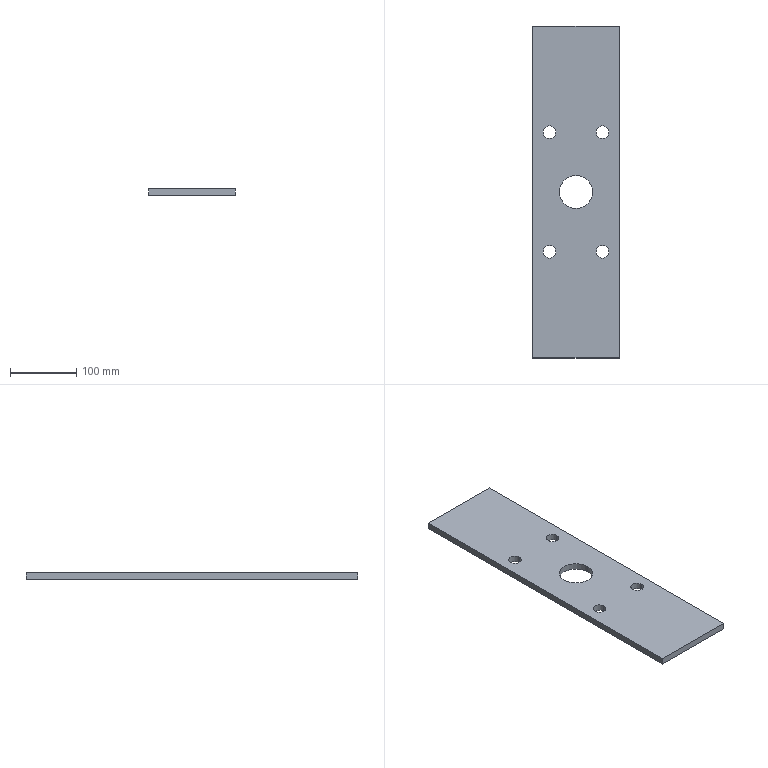Part | STEP file | MYT-A01-P28 | 1 solid | 16 faces | box 130 x 500 x 10 mm | volume 619024 mm3 | cylinder 10 | plane 6 | commonest cylinder face diameters 19 x8 50 x2
STEP:
#1=CARTESIAN_POINT('',(30.5,90.,0.));
#2=VERTEX_POINT('',#1);
#3=CARTESIAN_POINT('',(49.5,90.,0.));
#4=VERTEX_POINT('',#3);
#5=CARTESIAN_POINT('',(40.,90.,0.));
#6=DIRECTION('',(0.,0.,1.));
#7=DIRECTION('',(-1.,0.,0.));
#8=AXIS2_PLACEMENT_3D('',#5,#6,#7);
#9=CIRCLE('',#8,9.5);
#10=EDGE_CURVE('',#2,#4,#9,.T.);
#11=ORIENTED_EDGE('',*,*,#10,.F.);
#12=CARTESIAN_POINT('',(30.5,90.,10.));
#13=VERTEX_POINT('',#12);
#14=CARTESIAN_POINT('',(30.5,90.,0.));
#15=DIRECTION('',(0.,0.,1.));
#16=VECTOR('',#15,1000.);
#17=LINE('',#14,#16);
#18=EDGE_CURVE('',#2,#13,#17,.T.);
#19=ORIENTED_EDGE('',*,*,#18,.T.);
#20=CARTESIAN_POINT('',(49.5,90.,10.));
#21=VERTEX_POINT('',#20);
#22=CARTESIAN_POINT('',(40.,90.,10.));
#23=DIRECTION('',(0.,0.,1.));
#24=DIRECTION('',(-1.,0.,0.));
#25=AXIS2_PLACEMENT_3D('',#22,#23,#24);
#26=CIRCLE('',#25,9.5);
#27=EDGE_CURVE('',#13,#21,#26,.T.);
#28=ORIENTED_EDGE('',*,*,#27,.T.);
#29=CARTESIAN_POINT('',(49.5,90.,0.));
#30=DIRECTION('',(0.,0.,1.));
#31=VECTOR('',#30,1000.);
#32=LINE('',#29,#31);
#33=EDGE_CURVE('',#4,#21,#32,.T.);
#34=ORIENTED_EDGE('',*,*,#33,.F.);
#35=EDGE_LOOP('',(#11,#19,#28,#34));
#36=FACE_OUTER_BOUND('',#35,.T.);
#37=CARTESIAN_POINT('',(40.,90.,0.));
#38=DIRECTION('',(0.,0.,1.));
#39=DIRECTION('',(1.,0.,0.));
#40=AXIS2_PLACEMENT_3D('',#37,#38,#39);
#41=CYLINDRICAL_SURFACE('',#40,9.5);
#42=ADVANCED_FACE('',(#36),#41,.F.);
#43=CARTESIAN_POINT('',(30.5,-90.,0.));
#44=VERTEX_POINT('',#43);
#45=CARTESIAN_POINT('',(49.5,-90.,0.));
#46=VERTEX_POINT('',#45);
#47=CARTESIAN_POINT('',(40.,-90.,0.));
#48=DIRECTION('',(0.,0.,1.));
#49=DIRECTION('',(-1.,0.,0.));
#50=AXIS2_PLACEMENT_3D('',#47,#48,#49);
#51=CIRCLE('',#50,9.5);
#52=EDGE_CURVE('',#44,#46,#51,.T.);
#53=ORIENTED_EDGE('',*,*,#52,.F.);
#54=CARTESIAN_POINT('',(30.5,-90.,10.));
#55=VERTEX_POINT('',#54);
#56=CARTESIAN_POINT('',(30.5,-90.,0.));
#57=DIRECTION('',(0.,0.,1.));
#58=VECTOR('',#57,1000.);
#59=LINE('',#56,#58);
#60=EDGE_CURVE('',#44,#55,#59,.T.);
#61=ORIENTED_EDGE('',*,*,#60,.T.);
#62=CARTESIAN_POINT('',(49.5,-90.,10.));
#63=VERTEX_POINT('',#62);
#64=CARTESIAN_POINT('',(40.,-90.,10.));
#65=DIRECTION('',(0.,0.,1.));
#66=DIRECTION('',(-1.,0.,0.));
#67=AXIS2_PLACEMENT_3D('',#64,#65,#66);
#68=CIRCLE('',#67,9.5);
#69=EDGE_CURVE('',#55,#63,#68,.T.);
#70=ORIENTED_EDGE('',*,*,#69,.T.);
#71=CARTESIAN_POINT('',(49.5,-90.,0.));
#72=DIRECTION('',(0.,0.,1.));
#73=VECTOR('',#72,1000.);
#74=LINE('',#71,#73);
#75=EDGE_CURVE('',#46,#63,#74,.T.);
#76=ORIENTED_EDGE('',*,*,#75,.F.);
#77=EDGE_LOOP('',(#53,#61,#70,#76));
#78=FACE_OUTER_BOUND('',#77,.T.);
#79=CARTESIAN_POINT('',(40.,-90.,0.));
#80=DIRECTION('',(0.,0.,1.));
#81=DIRECTION('',(1.,0.,0.));
#82=AXIS2_PLACEMENT_3D('',#79,#80,#81);
#83=CYLINDRICAL_SURFACE('',#82,9.5);
#84=ADVANCED_FACE('',(#78),#83,.F.);
#85=CARTESIAN_POINT('',(-49.5,-90.,0.));
#86=VERTEX_POINT('',#85);
#87=CARTESIAN_POINT('',(-30.5,-90.,0.));
#88=VERTEX_POINT('',#87);
#89=CARTESIAN_POINT('',(-40.,-90.,0.));
#90=DIRECTION('',(0.,0.,1.));
#91=DIRECTION('',(1.,0.,0.));
#92=AXIS2_PLACEMENT_3D('',#89,#90,#91);
#93=CIRCLE('',#92,9.5);
#94=EDGE_CURVE('',#86,#88,#93,.T.);
#95=ORIENTED_EDGE('',*,*,#94,.F.);
#96=CARTESIAN_POINT('',(-49.5,-90.,10.));
#97=VERTEX_POINT('',#96);
#98=CARTESIAN_POINT('',(-49.5,-90.,0.));
#99=DIRECTION('',(0.,0.,1.));
#100=VECTOR('',#99,1000.);
#101=LINE('',#98,#100);
#102=EDGE_CURVE('',#86,#97,#101,.T.);
#103=ORIENTED_EDGE('',*,*,#102,.T.);
#104=CARTESIAN_POINT('',(-30.5,-90.,10.));
#105=VERTEX_POINT('',#104);
#106=CARTESIAN_POINT('',(-40.,-90.,10.));
#107=DIRECTION('',(0.,0.,1.));
#108=DIRECTION('',(1.,0.,0.));
#109=AXIS2_PLACEMENT_3D('',#106,#107,#108);
#110=CIRCLE('',#109,9.5);
#111=EDGE_CURVE('',#97,#105,#110,.T.);
#112=ORIENTED_EDGE('',*,*,#111,.T.);
#113=CARTESIAN_POINT('',(-30.5,-90.,0.));
#114=DIRECTION('',(0.,0.,1.));
#115=VECTOR('',#114,1000.);
#116=LINE('',#113,#115);
#117=EDGE_CURVE('',#88,#105,#116,.T.);
#118=ORIENTED_EDGE('',*,*,#117,.F.);
#119=EDGE_LOOP('',(#95,#103,#112,#118));
#120=FACE_OUTER_BOUND('',#119,.T.);
#121=CARTESIAN_POINT('',(-40.,-90.,0.));
#122=DIRECTION('',(0.,0.,1.));
#123=DIRECTION('',(1.,0.,0.));
#124=AXIS2_PLACEMENT_3D('',#121,#122,#123);
#125=CYLINDRICAL_SURFACE('',#124,9.5);
#126=ADVANCED_FACE('',(#120),#125,.F.);
#127=CARTESIAN_POINT('',(-49.5,90.,0.));
#128=VERTEX_POINT('',#127);
#129=CARTESIAN_POINT('',(-30.5,90.,0.));
#130=VERTEX_POINT('',#129);
#131=CARTESIAN_POINT('',(-40.,90.,0.));
#132=DIRECTION('',(0.,0.,1.));
#133=DIRECTION('',(1.,0.,0.));
#134=AXIS2_PLACEMENT_3D('',#131,#132,#133);
#135=CIRCLE('',#134,9.5);
#136=EDGE_CURVE('',#128,#130,#135,.T.);
#137=ORIENTED_EDGE('',*,*,#136,.F.);
#138=CARTESIAN_POINT('',(-49.5,90.,10.));
#139=VERTEX_POINT('',#138);
#140=CARTESIAN_POINT('',(-49.5,90.,0.));
#141=DIRECTION('',(0.,0.,1.));
#142=VECTOR('',#141,1000.);
#143=LINE('',#140,#142);
#144=EDGE_CURVE('',#128,#139,#143,.T.);
#145=ORIENTED_EDGE('',*,*,#144,.T.);
#146=CARTESIAN_POINT('',(-30.5,90.,10.));
#147=VERTEX_POINT('',#146);
#148=CARTESIAN_POINT('',(-40.,90.,10.));
#149=DIRECTION('',(0.,0.,1.));
#150=DIRECTION('',(1.,0.,0.));
#151=AXIS2_PLACEMENT_3D('',#148,#149,#150);
#152=CIRCLE('',#151,9.5);
#153=EDGE_CURVE('',#139,#147,#152,.T.);
#154=ORIENTED_EDGE('',*,*,#153,.T.);
#155=CARTESIAN_POINT('',(-30.5,90.,0.));
#156=DIRECTION('',(0.,0.,1.));
#157=VECTOR('',#156,1000.);
#158=LINE('',#155,#157);
#159=EDGE_CURVE('',#130,#147,#158,.T.);
#160=ORIENTED_EDGE('',*,*,#159,.F.);
#161=EDGE_LOOP('',(#137,#145,#154,#160));
#162=FACE_OUTER_BOUND('',#161,.T.);
#163=CARTESIAN_POINT('',(-40.,90.,0.));
#164=DIRECTION('',(0.,0.,1.));
#165=DIRECTION('',(1.,0.,0.));
#166=AXIS2_PLACEMENT_3D('',#163,#164,#165);
#167=CYLINDRICAL_SURFACE('',#166,9.5);
#168=ADVANCED_FACE('',(#162),#167,.F.);
#169=CARTESIAN_POINT('',(-25.,0.,0.));
#170=VERTEX_POINT('',#169);
#171=CARTESIAN_POINT('',(25.,0.,0.));
#172=VERTEX_POINT('',#171);
#173=CARTESIAN_POINT('',(0.,0.,0.));
#174=DIRECTION('',(0.,0.,1.));
#175=DIRECTION('',(1.,0.,0.));
#176=AXIS2_PLACEMENT_3D('',#173,#174,#175);
#177=CIRCLE('',#176,25.);
#178=EDGE_CURVE('',#170,#172,#177,.T.);
#179=ORIENTED_EDGE('',*,*,#178,.F.);
#180=CARTESIAN_POINT('',(-25.,0.,10.));
#181=VERTEX_POINT('',#180);
#182=CARTESIAN_POINT('',(-25.,0.,0.));
#183=DIRECTION('',(0.,0.,1.));
#184=VECTOR('',#183,1000.);
#185=LINE('',#182,#184);
#186=EDGE_CURVE('',#170,#181,#185,.T.);
#187=ORIENTED_EDGE('',*,*,#186,.T.);
#188=CARTESIAN_POINT('',(25.,0.,10.));
#189=VERTEX_POINT('',#188);
#190=CARTESIAN_POINT('',(0.,0.,10.));
#191=DIRECTION('',(0.,0.,1.));
#192=DIRECTION('',(1.,0.,0.));
#193=AXIS2_PLACEMENT_3D('',#190,#191,#192);
#194=CIRCLE('',#193,25.);
#195=EDGE_CURVE('',#181,#189,#194,.T.);
#196=ORIENTED_EDGE('',*,*,#195,.T.);
#197=CARTESIAN_POINT('',(25.,0.,0.));
#198=DIRECTION('',(0.,0.,1.));
#199=VECTOR('',#198,1000.);
#200=LINE('',#197,#199);
#201=EDGE_CURVE('',#172,#189,#200,.T.);
#202=ORIENTED_EDGE('',*,*,#201,.F.);
#203=EDGE_LOOP('',(#179,#187,#196,#202));
#204=FACE_OUTER_BOUND('',#203,.T.);
#205=CARTESIAN_POINT('',(0.,0.,0.));
#206=DIRECTION('',(0.,0.,1.));
#207=DIRECTION('',(1.,0.,0.));
#208=AXIS2_PLACEMENT_3D('',#205,#206,#207);
#209=CYLINDRICAL_SURFACE('',#208,25.);
#210=ADVANCED_FACE('',(#204),#209,.F.);
#211=CARTESIAN_POINT('',(65.,-250.,0.));
#212=VERTEX_POINT('',#211);
#213=CARTESIAN_POINT('',(65.,250.,0.));
#214=VERTEX_POINT('',#213);
#215=CARTESIAN_POINT('',(65.,250.,0.));
#216=DIRECTION('',(0.,1.,0.));
#217=VECTOR('',#216,1000.);
#218=LINE('',#215,#217);
#219=EDGE_CURVE('',#212,#214,#218,.T.);
#220=ORIENTED_EDGE('',*,*,#219,.T.);
#221=CARTESIAN_POINT('',(65.,250.,10.));
#222=VERTEX_POINT('',#221);
#223=CARTESIAN_POINT('',(65.,250.,10.));
#224=DIRECTION('',(0.,0.,-1.));
#225=VECTOR('',#224,1000.);
#226=LINE('',#223,#225);
#227=EDGE_CURVE('',#222,#214,#226,.T.);
#228=ORIENTED_EDGE('',*,*,#227,.F.);
#229=CARTESIAN_POINT('',(65.,-250.,10.));
#230=VERTEX_POINT('',#229);
#231=CARTESIAN_POINT('',(65.,250.,10.));
#232=DIRECTION('',(0.,1.,0.));
#233=VECTOR('',#232,1000.);
#234=LINE('',#231,#233);
#235=EDGE_CURVE('',#230,#222,#234,.T.);
#236=ORIENTED_EDGE('',*,*,#235,.F.);
#237=CARTESIAN_POINT('',(65.,-250.,10.));
#238=DIRECTION('',(0.,0.,-1.));
#239=VECTOR('',#238,1000.);
#240=LINE('',#237,#239);
#241=EDGE_CURVE('',#230,#212,#240,.T.);
#242=ORIENTED_EDGE('',*,*,#241,.T.);
#243=EDGE_LOOP('',(#220,#228,#236,#242));
#244=FACE_OUTER_BOUND('',#243,.T.);
#245=CARTESIAN_POINT('',(65.,250.,10.));
#246=DIRECTION('',(-1.,0.,0.));
#247=DIRECTION('',(0.,-1.,0.));
#248=AXIS2_PLACEMENT_3D('',#245,#246,#247);
#249=PLANE('',#248);
#250=ADVANCED_FACE('',(#244),#249,.F.);
#251=CARTESIAN_POINT('',(-65.,250.,0.));
#252=VERTEX_POINT('',#251);
#253=CARTESIAN_POINT('',(-65.,250.,0.));
#254=DIRECTION('',(-1.,0.,0.));
#255=VECTOR('',#254,1000.);
#256=LINE('',#253,#255);
#257=EDGE_CURVE('',#214,#252,#256,.T.);
#258=ORIENTED_EDGE('',*,*,#257,.T.);
#259=CARTESIAN_POINT('',(-65.,250.,10.));
#260=VERTEX_POINT('',#259);
#261=CARTESIAN_POINT('',(-65.,250.,10.));
#262=DIRECTION('',(0.,0.,-1.));
#263=VECTOR('',#262,1000.);
#264=LINE('',#261,#263);
#265=EDGE_CURVE('',#260,#252,#264,.T.);
#266=ORIENTED_EDGE('',*,*,#265,.F.);
#267=CARTESIAN_POINT('',(-65.,250.,10.));
#268=DIRECTION('',(-1.,0.,0.));
#269=VECTOR('',#268,1000.);
#270=LINE('',#267,#269);
#271=EDGE_CURVE('',#222,#260,#270,.T.);
#272=ORIENTED_EDGE('',*,*,#271,.F.);
#273=ORIENTED_EDGE('',*,*,#227,.T.);
#274=EDGE_LOOP('',(#258,#266,#272,#273));
#275=FACE_OUTER_BOUND('',#274,.T.);
#276=CARTESIAN_POINT('',(-65.,250.,10.));
#277=DIRECTION('',(0.,-1.,0.));
#278=DIRECTION('',(0.,0.,-1.));
#279=AXIS2_PLACEMENT_3D('',#276,#277,#278);
#280=PLANE('',#279);
#281=ADVANCED_FACE('',(#275),#280,.F.);
#282=CARTESIAN_POINT('',(-65.,-250.,0.));
#283=VERTEX_POINT('',#282);
#284=CARTESIAN_POINT('',(-65.,250.,0.));
#285=DIRECTION('',(0.,-1.,0.));
#286=VECTOR('',#285,1000.);
#287=LINE('',#284,#286);
#288=EDGE_CURVE('',#252,#283,#287,.T.);
#289=ORIENTED_EDGE('',*,*,#288,.T.);
#290=CARTESIAN_POINT('',(-65.,-250.,10.));
#291=VERTEX_POINT('',#290);
#292=CARTESIAN_POINT('',(-65.,-250.,10.));
#293=DIRECTION('',(0.,0.,-1.));
#294=VECTOR('',#293,1000.);
#295=LINE('',#292,#294);
#296=EDGE_CURVE('',#291,#283,#295,.T.);
#297=ORIENTED_EDGE('',*,*,#296,.F.);
#298=CARTESIAN_POINT('',(-65.,250.,10.));
#299=DIRECTION('',(0.,-1.,0.));
#300=VECTOR('',#299,1000.);
#301=LINE('',#298,#300);
#302=EDGE_CURVE('',#260,#291,#301,.T.);
#303=ORIENTED_EDGE('',*,*,#302,.F.);
#304=ORIENTED_EDGE('',*,*,#265,.T.);
#305=EDGE_LOOP('',(#289,#297,#303,#304));
#306=FACE_OUTER_BOUND('',#305,.T.);
#307=CARTESIAN_POINT('',(-65.,250.,10.));
#308=DIRECTION('',(1.,0.,0.));
#309=DIRECTION('',(0.,1.,0.));
#310=AXIS2_PLACEMENT_3D('',#307,#308,#309);
#311=PLANE('',#310);
#312=ADVANCED_FACE('',(#306),#311,.F.);
#313=CARTESIAN_POINT('',(-65.,-250.,0.));
#314=DIRECTION('',(1.,0.,0.));
#315=VECTOR('',#314,1000.);
#316=LINE('',#313,#315);
#317=EDGE_CURVE('',#283,#212,#316,.T.);
#318=ORIENTED_EDGE('',*,*,#317,.T.);
#319=ORIENTED_EDGE('',*,*,#241,.F.);
#320=CARTESIAN_POINT('',(-65.,-250.,10.));
#321=DIRECTION('',(1.,0.,0.));
#322=VECTOR('',#321,1000.);
#323=LINE('',#320,#322);
#324=EDGE_CURVE('',#291,#230,#323,.T.);
#325=ORIENTED_EDGE('',*,*,#324,.F.);
#326=ORIENTED_EDGE('',*,*,#296,.T.);
#327=EDGE_LOOP('',(#318,#319,#325,#326));
#328=FACE_OUTER_BOUND('',#327,.T.);
#329=CARTESIAN_POINT('',(-65.,-250.,10.));
#330=DIRECTION('',(0.,1.,0.));
#331=DIRECTION('',(0.,0.,1.));
#332=AXIS2_PLACEMENT_3D('',#329,#330,#331);
#333=PLANE('',#332);
#334=ADVANCED_FACE('',(#328),#333,.F.);
#335=CARTESIAN_POINT('',(40.,90.,10.));
#336=DIRECTION('',(0.,0.,1.));
#337=DIRECTION('',(-1.,0.,0.));
#338=AXIS2_PLACEMENT_3D('',#335,#336,#337);
#339=CIRCLE('',#338,9.5);
#340=EDGE_CURVE('',#21,#13,#339,.T.);
#341=ORIENTED_EDGE('',*,*,#340,.F.);
#342=ORIENTED_EDGE('',*,*,#27,.F.);
#343=EDGE_LOOP('',(#341,#342));
#344=FACE_BOUND('',#343,.T.);
#345=CARTESIAN_POINT('',(40.,-90.,10.));
#346=DIRECTION('',(0.,0.,1.));
#347=DIRECTION('',(-1.,0.,0.));
#348=AXIS2_PLACEMENT_3D('',#345,#346,#347);
#349=CIRCLE('',#348,9.5);
#350=EDGE_CURVE('',#63,#55,#349,.T.);
#351=ORIENTED_EDGE('',*,*,#350,.F.);
#352=ORIENTED_EDGE('',*,*,#69,.F.);
#353=EDGE_LOOP('',(#351,#352));
#354=FACE_BOUND('',#353,.T.);
#355=CARTESIAN_POINT('',(-40.,-90.,10.));
#356=DIRECTION('',(0.,0.,1.));
#357=DIRECTION('',(1.,0.,0.));
#358=AXIS2_PLACEMENT_3D('',#355,#356,#357);
#359=CIRCLE('',#358,9.5);
#360=EDGE_CURVE('',#105,#97,#359,.T.);
#361=ORIENTED_EDGE('',*,*,#360,.F.);
#362=ORIENTED_EDGE('',*,*,#111,.F.);
#363=EDGE_LOOP('',(#361,#362));
#364=FACE_BOUND('',#363,.T.);
#365=CARTESIAN_POINT('',(-40.,90.,10.));
#366=DIRECTION('',(0.,0.,1.));
#367=DIRECTION('',(1.,0.,0.));
#368=AXIS2_PLACEMENT_3D('',#365,#366,#367);
#369=CIRCLE('',#368,9.5);
#370=EDGE_CURVE('',#147,#139,#369,.T.);
#371=ORIENTED_EDGE('',*,*,#370,.F.);
#372=ORIENTED_EDGE('',*,*,#153,.F.);
#373=EDGE_LOOP('',(#371,#372));
#374=FACE_BOUND('',#373,.T.);
#375=CARTESIAN_POINT('',(0.,0.,10.));
#376=DIRECTION('',(0.,0.,1.));
#377=DIRECTION('',(1.,0.,0.));
#378=AXIS2_PLACEMENT_3D('',#375,#376,#377);
#379=CIRCLE('',#378,25.);
#380=EDGE_CURVE('',#189,#181,#379,.T.);
#381=ORIENTED_EDGE('',*,*,#380,.F.);
#382=ORIENTED_EDGE('',*,*,#195,.F.);
#383=EDGE_LOOP('',(#381,#382));
#384=FACE_BOUND('',#383,.T.);
#385=ORIENTED_EDGE('',*,*,#235,.T.);
#386=ORIENTED_EDGE('',*,*,#271,.T.);
#387=ORIENTED_EDGE('',*,*,#302,.T.);
#388=ORIENTED_EDGE('',*,*,#324,.T.);
#389=EDGE_LOOP('',(#385,#386,#387,#388));
#390=FACE_OUTER_BOUND('',#389,.T.);
#391=CARTESIAN_POINT('',(0.,0.,10.));
#392=DIRECTION('',(0.,0.,1.));
#393=DIRECTION('',(1.,0.,0.));
#394=AXIS2_PLACEMENT_3D('',#391,#392,#393);
#395=PLANE('',#394);
#396=ADVANCED_FACE('',(#344,#354,#364,#374,#384,#390),#395,.T.);
#397=CARTESIAN_POINT('',(40.,90.,0.));
#398=DIRECTION('',(0.,0.,1.));
#399=DIRECTION('',(-1.,0.,0.));
#400=AXIS2_PLACEMENT_3D('',#397,#398,#399);
#401=CIRCLE('',#400,9.5);
#402=EDGE_CURVE('',#4,#2,#401,.T.);
#403=ORIENTED_EDGE('',*,*,#402,.T.);
#404=ORIENTED_EDGE('',*,*,#10,.T.);
#405=EDGE_LOOP('',(#403,#404));
#406=FACE_BOUND('',#405,.T.);
#407=CARTESIAN_POINT('',(40.,-90.,0.));
#408=DIRECTION('',(0.,0.,1.));
#409=DIRECTION('',(-1.,0.,0.));
#410=AXIS2_PLACEMENT_3D('',#407,#408,#409);
#411=CIRCLE('',#410,9.5);
#412=EDGE_CURVE('',#46,#44,#411,.T.);
#413=ORIENTED_EDGE('',*,*,#412,.T.);
#414=ORIENTED_EDGE('',*,*,#52,.T.);
#415=EDGE_LOOP('',(#413,#414));
#416=FACE_BOUND('',#415,.T.);
#417=CARTESIAN_POINT('',(-40.,-90.,0.));
#418=DIRECTION('',(0.,0.,1.));
#419=DIRECTION('',(1.,0.,0.));
#420=AXIS2_PLACEMENT_3D('',#417,#418,#419);
#421=CIRCLE('',#420,9.5);
#422=EDGE_CURVE('',#88,#86,#421,.T.);
#423=ORIENTED_EDGE('',*,*,#422,.T.);
#424=ORIENTED_EDGE('',*,*,#94,.T.);
#425=EDGE_LOOP('',(#423,#424));
#426=FACE_BOUND('',#425,.T.);
#427=CARTESIAN_POINT('',(-40.,90.,0.));
#428=DIRECTION('',(0.,0.,1.));
#429=DIRECTION('',(1.,0.,0.));
#430=AXIS2_PLACEMENT_3D('',#427,#428,#429);
#431=CIRCLE('',#430,9.5);
#432=EDGE_CURVE('',#130,#128,#431,.T.);
#433=ORIENTED_EDGE('',*,*,#432,.T.);
#434=ORIENTED_EDGE('',*,*,#136,.T.);
#435=EDGE_LOOP('',(#433,#434));
#436=FACE_BOUND('',#435,.T.);
#437=CARTESIAN_POINT('',(0.,0.,0.));
#438=DIRECTION('',(0.,0.,1.));
#439=DIRECTION('',(1.,0.,0.));
#440=AXIS2_PLACEMENT_3D('',#437,#438,#439);
#441=CIRCLE('',#440,25.);
#442=EDGE_CURVE('',#172,#170,#441,.T.);
#443=ORIENTED_EDGE('',*,*,#442,.T.);
#444=ORIENTED_EDGE('',*,*,#178,.T.);
#445=EDGE_LOOP('',(#443,#444));
#446=FACE_BOUND('',#445,.T.);
#447=ORIENTED_EDGE('',*,*,#219,.F.);
#448=ORIENTED_EDGE('',*,*,#317,.F.);
#449=ORIENTED_EDGE('',*,*,#288,.F.);
#450=ORIENTED_EDGE('',*,*,#257,.F.);
#451=EDGE_LOOP('',(#447,#448,#449,#450));
#452=FACE_OUTER_BOUND('',#451,.T.);
#453=CARTESIAN_POINT('',(0.,0.,0.));
#454=DIRECTION('',(0.,0.,1.));
#455=DIRECTION('',(1.,0.,0.));
#456=AXIS2_PLACEMENT_3D('',#453,#454,#455);
#457=PLANE('',#456);
#458=ADVANCED_FACE('',(#406,#416,#426,#436,#446,#452),#457,.F.);
#459=ORIENTED_EDGE('',*,*,#186,.F.);
#460=ORIENTED_EDGE('',*,*,#442,.F.);
#461=ORIENTED_EDGE('',*,*,#201,.T.);
#462=ORIENTED_EDGE('',*,*,#380,.T.);
#463=EDGE_LOOP('',(#459,#460,#461,#462));
#464=FACE_OUTER_BOUND('',#463,.T.);
#465=CARTESIAN_POINT('',(0.,0.,0.));
#466=DIRECTION('',(0.,0.,1.));
#467=DIRECTION('',(1.,0.,0.));
#468=AXIS2_PLACEMENT_3D('',#465,#466,#467);
#469=CYLINDRICAL_SURFACE('',#468,25.);
#470=ADVANCED_FACE('',(#464),#469,.F.);
#471=ORIENTED_EDGE('',*,*,#144,.F.);
#472=ORIENTED_EDGE('',*,*,#432,.F.);
#473=ORIENTED_EDGE('',*,*,#159,.T.);
#474=ORIENTED_EDGE('',*,*,#370,.T.);
#475=EDGE_LOOP('',(#471,#472,#473,#474));
#476=FACE_OUTER_BOUND('',#475,.T.);
#477=CARTESIAN_POINT('',(-40.,90.,0.));
#478=DIRECTION('',(0.,0.,1.));
#479=DIRECTION('',(1.,0.,0.));
#480=AXIS2_PLACEMENT_3D('',#477,#478,#479);
#481=CYLINDRICAL_SURFACE('',#480,9.5);
#482=ADVANCED_FACE('',(#476),#481,.F.);
#483=ORIENTED_EDGE('',*,*,#102,.F.);
#484=ORIENTED_EDGE('',*,*,#422,.F.);
#485=ORIENTED_EDGE('',*,*,#117,.T.);
#486=ORIENTED_EDGE('',*,*,#360,.T.);
#487=EDGE_LOOP('',(#483,#484,#485,#486));
#488=FACE_OUTER_BOUND('',#487,.T.);
#489=CARTESIAN_POINT('',(-40.,-90.,0.));
#490=DIRECTION('',(0.,0.,1.));
#491=DIRECTION('',(1.,0.,0.));
#492=AXIS2_PLACEMENT_3D('',#489,#490,#491);
#493=CYLINDRICAL_SURFACE('',#492,9.5);
#494=ADVANCED_FACE('',(#488),#493,.F.);
#495=ORIENTED_EDGE('',*,*,#60,.F.);
#496=ORIENTED_EDGE('',*,*,#412,.F.);
#497=ORIENTED_EDGE('',*,*,#75,.T.);
#498=ORIENTED_EDGE('',*,*,#350,.T.);
#499=EDGE_LOOP('',(#495,#496,#497,#498));
#500=FACE_OUTER_BOUND('',#499,.T.);
#501=CARTESIAN_POINT('',(40.,-90.,0.));
#502=DIRECTION('',(0.,0.,1.));
#503=DIRECTION('',(1.,0.,0.));
#504=AXIS2_PLACEMENT_3D('',#501,#502,#503);
#505=CYLINDRICAL_SURFACE('',#504,9.5);
#506=ADVANCED_FACE('',(#500),#505,.F.);
#507=ORIENTED_EDGE('',*,*,#18,.F.);
#508=ORIENTED_EDGE('',*,*,#402,.F.);
#509=ORIENTED_EDGE('',*,*,#33,.T.);
#510=ORIENTED_EDGE('',*,*,#340,.T.);
#511=EDGE_LOOP('',(#507,#508,#509,#510));
#512=FACE_OUTER_BOUND('',#511,.T.);
#513=CARTESIAN_POINT('',(40.,90.,0.));
#514=DIRECTION('',(0.,0.,1.));
#515=DIRECTION('',(1.,0.,0.));
#516=AXIS2_PLACEMENT_3D('',#513,#514,#515);
#517=CYLINDRICAL_SURFACE('',#516,9.5);
#518=ADVANCED_FACE('',(#512),#517,.F.);
#519=CLOSED_SHELL('',(#42,#84,#126,#168,#210,#250,#281,#312,#334,#396,#458,#470,#482,#494,#506,#518));
#520=MANIFOLD_SOLID_BREP('',#519);
#521=CARTESIAN_POINT('',(0.,0.,0.));
#522=DIRECTION('',(0.,0.,1.));
#523=DIRECTION('',(1.,0.,0.));
#524=AXIS2_PLACEMENT_3D('',#521,#522,#523);
#525=(LENGTH_UNIT()NAMED_UNIT(*)SI_UNIT(.MILLI.,.METRE.));
#526=UNCERTAINTY_MEASURE_WITH_UNIT(LENGTH_MEASURE(0.00001),#525,'','');
#527=(NAMED_UNIT(*)PLANE_ANGLE_UNIT()SI_UNIT($,.RADIAN.));
#528=(NAMED_UNIT(*)SI_UNIT($,.STERADIAN.)SOLID_ANGLE_UNIT());
#529=(GEOMETRIC_REPRESENTATION_CONTEXT(3)GLOBAL_UNCERTAINTY_ASSIGNED_CONTEXT((#526))GLOBAL_UNIT_ASSIGNED_CONTEXT((#525,#527,#528))REPRESENTATION_CONTEXT('',''));
#530=ADVANCED_BREP_SHAPE_REPRESENTATION('',(#520,#524),#529);